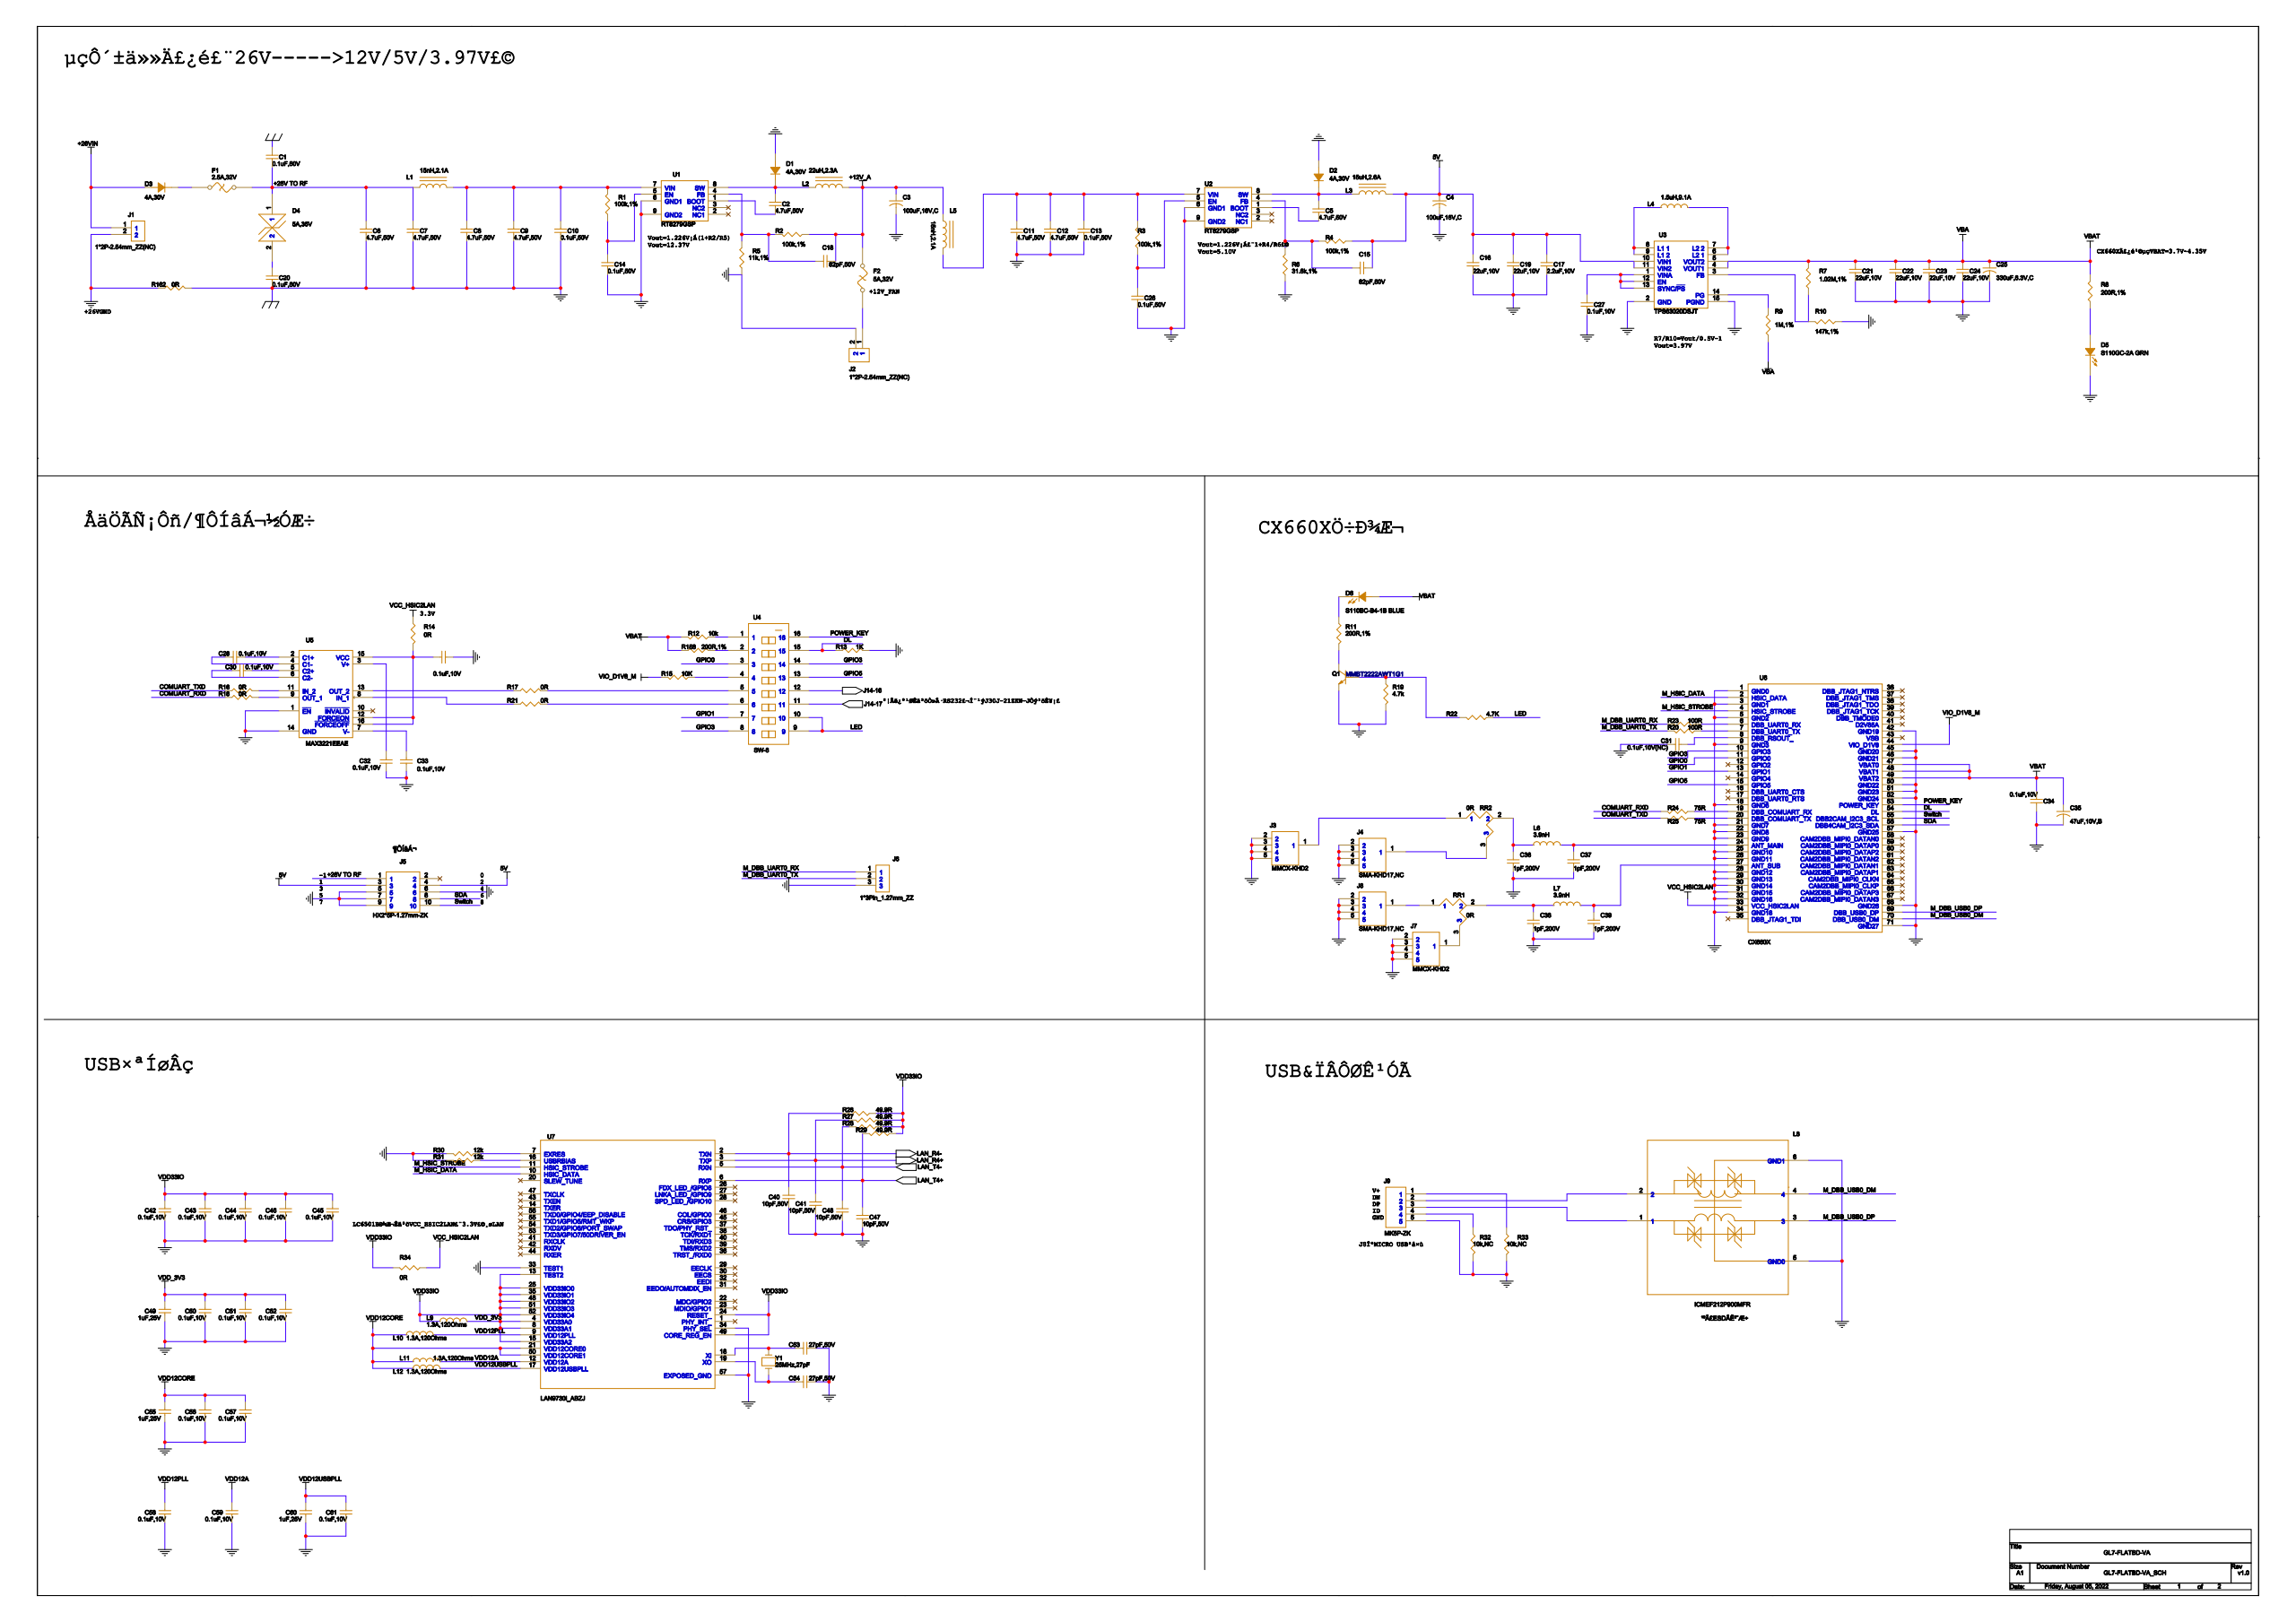Circuit board | Cadence Allegro | 338 parts | 273 nets | one sheet of the schematic
Parts on this sheet (reference | value | footprint):
C1 | 0.1uF,50V | 0402C
C2 | 4.7uF,50V | 0805C
C3 | 100uF,16V,C | CA45C
C4 | 100uF,16V,C | CA45C
C5 | 4.7uF,50V | 0805C
C6 | 4.7uF,50V | 0805C
C7 | 4.7uF,50V | 0805C
C8 | 4.7uF,50V | 0805C
C9 | 4.7uF,50V | 0805C
C10 | 0.1uF,50V | 0402C
C11 | 4.7uF,50V | 0805C
C12 | 4.7uF,50V | 0805C
C13 | 0.1uF,50V | 0402C
C14 | 0.1uF,50V | 0402C
C15 | 82pF,50V | 0402C
C16 | 22uF,10V | 0603C
C17 | 2.2uF,10V | 0402C
C18 | 82pF,50V | 0402C
C19 | 22uF,10V | 0603C
C20 | 0.1uF,50V | 0402C
C21 | 22uF,10V | 0603C
C22 | 22uF,10V | 0603C
C23 | 22uF,10V | 0603C
C24 | 22uF,10V | 0603C
C25 | 330uF,6.3V,C | CA45C
C26 | 0.1uF,50V | 0402C
C27 | 0.1uF,10V | 0402C
C28 | 0.1uF,10V | 0402C
C30 | 0.1uF,10V | 0402C
C31 | 0.1uF,10V(NC) | 0402C
C32 | 0.1uF,10V | 0402C
C33 | 0.1uF,10V | 0402C
C34 | 0.1uF,10V | 0402C
C35 | 47uF,10V,B | CAKB
C36 | 1pF,200V | 0402C
C37 | 1pF,200V | 0402C
C38 | 1pF,200V | 0402C
C39 | 1pF,200V | 0402C
C40 | 10pF,50V | 0402C
C41 | 10pF,50V | 0402C
C42 | 0.1uF,10V | 0402C
C43 | 0.1uF,10V | 0402C
C44 | 0.1uF,10V | 0402C
C45 | 0.1uF,10V | 0402C
C46 | 0.1uF,10V | 0402C
C47 | 10pF,50V | 0402C
C48 | 10pF,50V | 0402C
C49 | 1uF,25V | 0402C
C50 | 0.1uF,10V | 0402C
C51 | 0.1uF,10V | 0402C
C52 | 0.1uF,10V | 0402C
C53 | 27pF,50V | 0402C
C54 | 27pF,50V | 0402C
C55 | 1uF,25V | 0402C
C56 | 0.1uF,10V | 0402C
C57 | 0.1uF,10V | 0402C
C58 | 0.1uF,10V | 0402C
C59 | 0.1uF,10V | 0402C
C60 | 1uF,25V | 0402C
C61 | 0.1uF,10V | 0402C
D1 | 4A,30V | DO_214AA
D2 | 4A,30V | DO_214AA
D3 | 4A,30V | DO_214AA
D4 | 5A,36V | DO_-214AA
D5 | S110GC-2A GRN | S110BC
D6 | S110BC-B4-1B BLUE | S110BC
F1 | 2.5A,32V | 1206
F2 | 5A,32V | SF-1206F500
J1 | 1*2P-2.54mm_ZZ(NC) | 2P54-1-2
J2 | 1*2P-2.54mm_ZZ(NC) | 2P54-1-2
J3 | MMCX-KHD2 | MMCX-KHD2
J4 | DOSIN-806-0331 | DOSIN-806-0331
J5 | HX2*5P-1.27mm-ZK | 1P27-2-5-L-SMT
J6 | 1*3Pin_1.27mm_ZZ | 1P27-1-3
J7 | MMCX-KHD2 | MMCX-KHD2
J8 | DOSIN-806-0331 | DOSIN-806-0331
J9 | MK5P-ZK | MICRO-USB_5_9
L1 | 15nH,2.1A | 0603L
L2 | 22uH,2.3A | WHC
L3 | 15uH,2.6A | WHC
L4 | 1.5uH,9.1A | 0603L
L5 | 15nH,2.1A | 0603L
L6 | 3.9nH | 0402L
L7 | 3.9nH | 0402L
L8 | ICMEF212P900MFR | ICT_ICMEF212P900MFR_S
L9 | 1.3A,120Ohms | 0402L
L10 | 1.3A,120Ohms | 0402L
L11 | 1.3A,120Ohms | 0402L
L12 | 1.3A,120Ohms | 0402L
Q1 | L14C1/TO | SOT-323
R1 | 100k,1% | 0402R
R2 | 100k,1% | 0402R
R3 | 100k,1% | 0402R
R4 | 100k,1% | 0402R
R5 | 11k,1% | 0402R
R6 | 31.6k,1% | 0402R
R7 | 1.02M,1% | 0402R
R8 | 200R,1% | 0402R
R9 | 1M,1% | 0402R
R10 | 147k,1% | 0402R
R11 | 200R | 0402R
R12 | 10k | 0402R
R13 | 1K | 0402R
R14 | 0R | 0402R
R15 | 10k | 0402R
R16 | 0R | 0402R
R17 | 0R | 0402R
R18 | 0R | 0402R
R19 | 4.7K | 0402R
R20 | 100R | 0402R
R21 | 0R | 0402R
R22 | 4.7K | 0402R
R23 | 100R | 0402R
R24 | 75R | 0402R
R25 | 75R | 0402R
R26 | 49.9R | 0402R
R27 | 49.9R | 0402R
R28 | 49.9R | 0402R
R29 | 49.9R | 0402R
R30 | 12k | 0402R
R31 | 12k | 0402R
R32 | 10k(NC) | 0402R
R33 | 10k(NC) | 0402R
R34 | 0R | 0402R
R158 | 200R | 0402R
R162 | 0R | 0805R
RR1 | 0R | 04022R
RR2 | 0R | 04022R
U1 | RT8279GSP | SOP8
U2 | RT8279GSP | SOP8
U3 | TPS63020DSJT | DSJ14_2P85X1P58
U4 | SW-8 | KE_BMKG
U5 | MAX3221EEAE | SSOP16
U6 | CX660X | LC6500_PAD_S
U7 | LAN9730i_ABZJ | SMSC_QFN_56_S
Y1 | 25MHz,27pF | ABM7-25MHZ
Nets of these parts (net: part-pin ...):
+26VGND: J1-2 R162-1
GND: C1-1 C3-2 C4-2 C6-2 C7-2 C8-2 C9-2 C10-2 C11-2 C12-2 C13-2 C14-2 C16-2 C17-2 C19-2 C20-2 C21-2 C22-2 C23-2 C24-2 C25-2 C26-2 C27-2 C31-1 C32-1 C33-1 C34-2 C35-2 C36-2 C37-2 C38-2 C39-2 C40-2 C41-2 C42-2 C43-2 C44-2 C45-2 C46-2 C47-2 C48-2 C49-2 C50-2 C51-2 C52-2 C53-2 C54-2 C55-2 C56-2 C57-2 C58-2 C59-2 C60-2 C61-2 D1-2 D2-2 D5-1 J2-2 J3-2 J3-3 J3-4 J3-5 J4-2 J4-3 J4-4 J4-5 J5-5 J5-6 J5-7 J5-9 J6-3 J7-2 J7-3 J7-4 J7-5 J8-2 J8-3 J8-4 J8-5 J9-5 L8-5 L8-6 Q1-1 R5-1 R6-1 R10-1 R13-2 R19-2 R30-2 R31-2 R32-2 R33-2 R162-2 U1-6 U1-9 U2-6 U2-9 U3-2 U3-15 U5-1 U5-14 U6-1 U6-3 U6-5 U6-9 U6-18 U6-21 U6-22 U6-23 U6-25 U6-26 U6-28 U6-29 U6-30 U6-31 U6-32 U6-34 U6-42 U6-45 U6-46 U6-50 U6-51 U6-52 U6-57 U6-68 U6-71 U7-33 U7-34 U7-57
N16881378: C2-1 D1-1 L2-1 U1-8
+12V_A: C3-1 C18-2 F2-2 L2-2 L5-1 R2-1
N16881807: C5-1 D2-1 L3-1 U2-8
5V: C4-1 C15-2 C16-1 C17-1 C19-1 L3-2 R4-1 U3-10 U3-11
VBA: C21-1 C22-1 C23-1 C24-1 C25-1 C34-1 C35-1 D6-2 R7-2 R8-2 R9-1 R12-2 R158-1 U3-4 U3-5 U6-47 U6-48 U6-49
M_DBB_UART0_RX_17471533: J6-1 R23-2
M_DBB_UART0_TX_17471536: J6-2 R20-2
N17666137: R12-1 U4-1
N16918768: R15-1 U4-4
VIO_D1V8_M: R15-2 U6-44
N17471590: R20-1 U6-7
N17471587: R23-1 U6-6
N16886631: D5-2 R8-1
N16901926: D6-1 R11-1
N17770006: J8-1 RR1-1
N17786541: J4-1 RR2-3
N16881392: C2-2 U1-1
N16880865: C14-1 R1-1 U1-5
N16881316: C18-1 R2-2 R5-2 U1-4
N16880616: C8-1 C9-1 C10-1 L1-2 R1-2 U1-7
N16881813: C5-2 U2-1
N16882192: C26-1 R3-1 U2-5
N16881787: C15-1 R4-2 R6-2 U2-4
N16881994: C11-1 C12-1 C13-1 L5-2 R3-2 U2-7
+26VIN: D3-2 J1-1
N16880400: D3-1 F1-1
+26V TO RF: C1-2 C6-1 C7-1 D4-1 F1-2 J5-1 L1-1
N17556645: C20-1 D4-2
N17638201: F2-1 J2-1
SWITCH: J5-10 U6-55
+5V: J5-3 J5-4
SDA: J5-8 U6-56
N16885620: L4-1 U3-6 U3-7
N16883441: L4-2 U3-8 U3-9
N16885672: R7-1 R10-2 U3-3
J14-16: U4-12
J14-17: U4-11
DL: R13-1 U4-15 U6-54
VDD33IO: C42-1 C43-1 C44-1 C45-1 C46-1 L9-2 R26-1 R27-1 R28-1 R29-1 R34-2 U7-13 U7-24 U7-25 U7-35 U7-48 U7-49 U7-51 U7-52
LAN_R4-: C40-1 R26-2 U7-2
LAN_R4+: C41-1 R27-2 U7-3
LAN_T4-: C48-1 R28-2 U7-5
LAN_T4+: C47-1 R29-2 U7-6
N16926650: R30-1 U7-7
N16927298: R31-1 U7-16
N16885982: R9-2 U3-14
LED: R22-1 U4-9 U4-10
GPIO5: U4-13 U6-15
GPIO3: U4-8 U4-14 U6-10
POWER_KEY: U4-16 U6-53
N17733086: R158-2 U4-2
GPIO0: U4-3 U6-11
N16918582: R17-2 U4-5
N16918572: R21-2 U4-6
GPIO1: U4-7 U6-13
N16897265: C37-1 L6-1 U6-24
N16900328: C39-1 L7-1 U6-27
N16898811: R24-1 U6-19
N16898817: R25-1 U6-20
N16898466: C31-2 U6-8
M_DBB_USB0_DM: L8-4 U6-70
M_DBB_USB0_DP: L8-3 U6-69
M_HSIC_DATA: U6-2 U7-10
M_HSIC_STROBE: U6-4 U7-11
VCC_HSIC2LAN: R14-1 R34-1 U6-33
N16923363: J9-3 L8-1
N16923360: J9-2 L8-2
N16883294: C27-1 U3-1 U3-12 U3-13
VDD12A: C59-1 L11-1 U7-12
VDD12CORE: C55-1 C56-1 C57-1 L10-2 L11-2 L12-2 U7-21 U7-50
VDD12PLL: C58-1 L10-1 U7-9
VDD12USBPLL: C60-1 C61-1 L12-1 U7-17
VDD_3V3: C49-1 C50-1 C51-1 C52-1 L9-1 U7-4 U7-8 U7-15
N16929314: C53-1 Y1-2 U7-18
N16929069: C54-1 Y1-1 U7-19
N16899432: J3-1 RR2-1
N16898912: C36-1 L6-2 RR2-2
N16900333: C38-1 L7-2 RR1-2
N173979642: J7-1 RR1-3
N17175739: C32-2 U5-3
N17159788: C28-1 U5-4
N16914520: C28-2 U5-2
N16976789: R14-2 U5-12 U5-15 U5-16
N16914538: C30-1 U5-6
N16914535: C30-2 U5-5
N17181357: C33-2 U5-7
N16901929: Q1-3 R11-2
COMUART_RXD: R18-1 R24-2
COMUART_TXD: R16-1 R25-2
N16922231: J9-4 R32-1
N16922679: J9-1 R33-1
N17468671: R21-1 U5-8
N17654246: R16-2 U5-11
N17654249: R18-2 U5-9
N17468345: R17-1 U5-13
N16901932: Q1-2 R19-1 R22-2